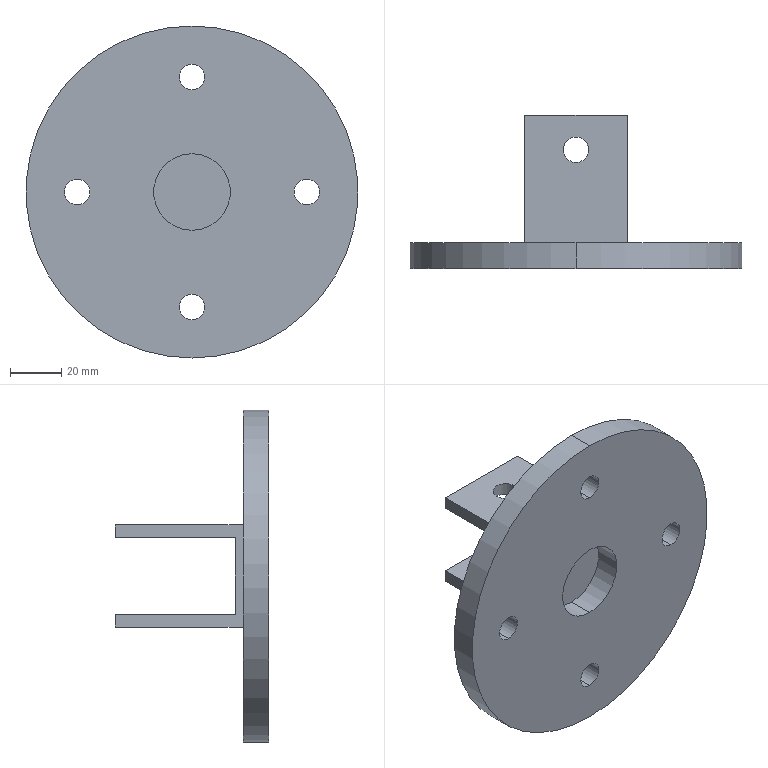Part | SolidWorks | features ICE 4, Extrusion 1 | 1 solid | 28 faces | box 130 x 60 x 130 mm | volume 145337 mm3 | cylinder 16 | plane 12 | commonest cylinder face diameters 10 x12 30 x2 130 x2
STEP:
#1=CARTESIAN_POINT('',(-5.,46.469,15.));
#2=VERTEX_POINT('',#1);
#3=CARTESIAN_POINT('',(5.,46.469,15.));
#4=VERTEX_POINT('',#3);
#5=CARTESIAN_POINT('',(0.,46.469,15.));
#6=DIRECTION('',(0.,0.,1.));
#7=DIRECTION('',(0.,-1.,0.));
#8=AXIS2_PLACEMENT_3D('',#5,#6,#7);
#9=CIRCLE('',#8,5.);
#10=EDGE_CURVE('',#2,#4,#9,.T.);
#11=ORIENTED_EDGE('',*,*,#10,.F.);
#12=CARTESIAN_POINT('',(-5.,46.469,20.));
#13=VERTEX_POINT('',#12);
#14=CARTESIAN_POINT('',(-5.,46.469,-65.));
#15=DIRECTION('',(0.,0.,1.));
#16=VECTOR('',#15,1000.);
#17=LINE('',#14,#16);
#18=EDGE_CURVE('',#2,#13,#17,.T.);
#19=ORIENTED_EDGE('',*,*,#18,.T.);
#20=CARTESIAN_POINT('',(5.,46.469,20.));
#21=VERTEX_POINT('',#20);
#22=CARTESIAN_POINT('',(0.,46.469,20.));
#23=DIRECTION('',(0.,0.,1.));
#24=DIRECTION('',(1.,0.,0.));
#25=AXIS2_PLACEMENT_3D('',#22,#23,#24);
#26=CIRCLE('',#25,5.);
#27=EDGE_CURVE('',#13,#21,#26,.T.);
#28=ORIENTED_EDGE('',*,*,#27,.T.);
#29=CARTESIAN_POINT('',(5.,46.469,-65.));
#30=DIRECTION('',(0.,0.,1.));
#31=VECTOR('',#30,1000.);
#32=LINE('',#29,#31);
#33=EDGE_CURVE('',#4,#21,#32,.T.);
#34=ORIENTED_EDGE('',*,*,#33,.F.);
#35=EDGE_LOOP('',(#11,#19,#28,#34));
#36=FACE_OUTER_BOUND('',#35,.T.);
#37=CARTESIAN_POINT('',(0.,46.469,-65.));
#38=DIRECTION('',(0.,0.,1.));
#39=DIRECTION('',(1.,0.,0.));
#40=AXIS2_PLACEMENT_3D('',#37,#38,#39);
#41=CYLINDRICAL_SURFACE('',#40,5.);
#42=ADVANCED_FACE('',(#36),#41,.F.);
#43=CARTESIAN_POINT('',(-5.,46.469,-20.));
#44=VERTEX_POINT('',#43);
#45=CARTESIAN_POINT('',(5.,46.469,-20.));
#46=VERTEX_POINT('',#45);
#47=CARTESIAN_POINT('',(0.,46.469,-20.));
#48=DIRECTION('',(0.,0.,1.));
#49=DIRECTION('',(1.,0.,0.));
#50=AXIS2_PLACEMENT_3D('',#47,#48,#49);
#51=CIRCLE('',#50,5.);
#52=EDGE_CURVE('',#44,#46,#51,.T.);
#53=ORIENTED_EDGE('',*,*,#52,.F.);
#54=CARTESIAN_POINT('',(-5.,46.469,-15.));
#55=VERTEX_POINT('',#54);
#56=CARTESIAN_POINT('',(-5.,46.469,-65.));
#57=DIRECTION('',(0.,0.,1.));
#58=VECTOR('',#57,1000.);
#59=LINE('',#56,#58);
#60=EDGE_CURVE('',#44,#55,#59,.T.);
#61=ORIENTED_EDGE('',*,*,#60,.T.);
#62=CARTESIAN_POINT('',(5.,46.469,-15.));
#63=VERTEX_POINT('',#62);
#64=CARTESIAN_POINT('',(0.,46.469,-15.));
#65=DIRECTION('',(0.,0.,-1.));
#66=DIRECTION('',(0.,1.,0.));
#67=AXIS2_PLACEMENT_3D('',#64,#65,#66);
#68=CIRCLE('',#67,5.);
#69=EDGE_CURVE('',#63,#55,#68,.T.);
#70=ORIENTED_EDGE('',*,*,#69,.F.);
#71=CARTESIAN_POINT('',(5.,46.469,-65.));
#72=DIRECTION('',(0.,0.,1.));
#73=VECTOR('',#72,1000.);
#74=LINE('',#71,#73);
#75=EDGE_CURVE('',#46,#63,#74,.T.);
#76=ORIENTED_EDGE('',*,*,#75,.F.);
#77=EDGE_LOOP('',(#53,#61,#70,#76));
#78=FACE_OUTER_BOUND('',#77,.T.);
#79=CARTESIAN_POINT('',(0.,46.469,-65.));
#80=DIRECTION('',(0.,0.,1.));
#81=DIRECTION('',(1.,0.,0.));
#82=AXIS2_PLACEMENT_3D('',#79,#80,#81);
#83=CYLINDRICAL_SURFACE('',#82,5.);
#84=ADVANCED_FACE('',(#78),#83,.F.);
#85=CARTESIAN_POINT('',(0.,0.,-50.));
#86=VERTEX_POINT('',#85);
#87=CARTESIAN_POINT('',(0.,0.,-40.));
#88=VERTEX_POINT('',#87);
#89=CARTESIAN_POINT('',(0.,0.,-45.));
#90=DIRECTION('',(0.,1.,0.));
#91=DIRECTION('',(0.,0.,1.));
#92=AXIS2_PLACEMENT_3D('',#89,#90,#91);
#93=CIRCLE('',#92,5.);
#94=EDGE_CURVE('',#86,#88,#93,.T.);
#95=ORIENTED_EDGE('',*,*,#94,.F.);
#96=CARTESIAN_POINT('',(0.,10.,-50.));
#97=VERTEX_POINT('',#96);
#98=CARTESIAN_POINT('',(0.,0.,-50.));
#99=DIRECTION('',(0.,1.,0.));
#100=VECTOR('',#99,1000.);
#101=LINE('',#98,#100);
#102=EDGE_CURVE('',#86,#97,#101,.T.);
#103=ORIENTED_EDGE('',*,*,#102,.T.);
#104=CARTESIAN_POINT('',(0.,10.,-40.));
#105=VERTEX_POINT('',#104);
#106=CARTESIAN_POINT('',(0.,10.,-45.));
#107=DIRECTION('',(0.,1.,0.));
#108=DIRECTION('',(0.,0.,1.));
#109=AXIS2_PLACEMENT_3D('',#106,#107,#108);
#110=CIRCLE('',#109,5.);
#111=EDGE_CURVE('',#97,#105,#110,.T.);
#112=ORIENTED_EDGE('',*,*,#111,.T.);
#113=CARTESIAN_POINT('',(0.,0.,-40.));
#114=DIRECTION('',(0.,1.,0.));
#115=VECTOR('',#114,1000.);
#116=LINE('',#113,#115);
#117=EDGE_CURVE('',#88,#105,#116,.T.);
#118=ORIENTED_EDGE('',*,*,#117,.F.);
#119=EDGE_LOOP('',(#95,#103,#112,#118));
#120=FACE_OUTER_BOUND('',#119,.T.);
#121=CARTESIAN_POINT('',(0.,0.,-45.));
#122=DIRECTION('',(0.,1.,0.));
#123=DIRECTION('',(0.,0.,1.));
#124=AXIS2_PLACEMENT_3D('',#121,#122,#123);
#125=CYLINDRICAL_SURFACE('',#124,5.);
#126=ADVANCED_FACE('',(#120),#125,.F.);
#127=CARTESIAN_POINT('',(45.,0.,-5.));
#128=VERTEX_POINT('',#127);
#129=CARTESIAN_POINT('',(45.,0.,5.));
#130=VERTEX_POINT('',#129);
#131=CARTESIAN_POINT('',(45.,0.,0.));
#132=DIRECTION('',(0.,1.,0.));
#133=DIRECTION('',(0.,0.,1.));
#134=AXIS2_PLACEMENT_3D('',#131,#132,#133);
#135=CIRCLE('',#134,5.);
#136=EDGE_CURVE('',#128,#130,#135,.T.);
#137=ORIENTED_EDGE('',*,*,#136,.F.);
#138=CARTESIAN_POINT('',(45.,10.,-5.));
#139=VERTEX_POINT('',#138);
#140=CARTESIAN_POINT('',(45.,0.,-5.));
#141=DIRECTION('',(0.,1.,0.));
#142=VECTOR('',#141,1000.);
#143=LINE('',#140,#142);
#144=EDGE_CURVE('',#128,#139,#143,.T.);
#145=ORIENTED_EDGE('',*,*,#144,.T.);
#146=CARTESIAN_POINT('',(45.,10.,5.));
#147=VERTEX_POINT('',#146);
#148=CARTESIAN_POINT('',(45.,10.,0.));
#149=DIRECTION('',(0.,1.,0.));
#150=DIRECTION('',(0.,0.,1.));
#151=AXIS2_PLACEMENT_3D('',#148,#149,#150);
#152=CIRCLE('',#151,5.);
#153=EDGE_CURVE('',#139,#147,#152,.T.);
#154=ORIENTED_EDGE('',*,*,#153,.T.);
#155=CARTESIAN_POINT('',(45.,0.,5.));
#156=DIRECTION('',(0.,1.,0.));
#157=VECTOR('',#156,1000.);
#158=LINE('',#155,#157);
#159=EDGE_CURVE('',#130,#147,#158,.T.);
#160=ORIENTED_EDGE('',*,*,#159,.F.);
#161=EDGE_LOOP('',(#137,#145,#154,#160));
#162=FACE_OUTER_BOUND('',#161,.T.);
#163=CARTESIAN_POINT('',(45.,0.,0.));
#164=DIRECTION('',(0.,1.,0.));
#165=DIRECTION('',(0.,0.,1.));
#166=AXIS2_PLACEMENT_3D('',#163,#164,#165);
#167=CYLINDRICAL_SURFACE('',#166,5.);
#168=ADVANCED_FACE('',(#162),#167,.F.);
#169=CARTESIAN_POINT('',(0.,0.,40.));
#170=VERTEX_POINT('',#169);
#171=CARTESIAN_POINT('',(0.,0.,50.));
#172=VERTEX_POINT('',#171);
#173=CARTESIAN_POINT('',(0.,0.,45.));
#174=DIRECTION('',(0.,1.,0.));
#175=DIRECTION('',(0.,0.,1.));
#176=AXIS2_PLACEMENT_3D('',#173,#174,#175);
#177=CIRCLE('',#176,5.);
#178=EDGE_CURVE('',#170,#172,#177,.T.);
#179=ORIENTED_EDGE('',*,*,#178,.F.);
#180=CARTESIAN_POINT('',(0.,10.,40.));
#181=VERTEX_POINT('',#180);
#182=CARTESIAN_POINT('',(0.,0.,40.));
#183=DIRECTION('',(0.,1.,0.));
#184=VECTOR('',#183,1000.);
#185=LINE('',#182,#184);
#186=EDGE_CURVE('',#170,#181,#185,.T.);
#187=ORIENTED_EDGE('',*,*,#186,.T.);
#188=CARTESIAN_POINT('',(0.,10.,50.));
#189=VERTEX_POINT('',#188);
#190=CARTESIAN_POINT('',(0.,10.,45.));
#191=DIRECTION('',(0.,1.,0.));
#192=DIRECTION('',(0.,0.,1.));
#193=AXIS2_PLACEMENT_3D('',#190,#191,#192);
#194=CIRCLE('',#193,5.);
#195=EDGE_CURVE('',#181,#189,#194,.T.);
#196=ORIENTED_EDGE('',*,*,#195,.T.);
#197=CARTESIAN_POINT('',(0.,0.,50.));
#198=DIRECTION('',(0.,1.,0.));
#199=VECTOR('',#198,1000.);
#200=LINE('',#197,#199);
#201=EDGE_CURVE('',#172,#189,#200,.T.);
#202=ORIENTED_EDGE('',*,*,#201,.F.);
#203=EDGE_LOOP('',(#179,#187,#196,#202));
#204=FACE_OUTER_BOUND('',#203,.T.);
#205=CARTESIAN_POINT('',(0.,0.,45.));
#206=DIRECTION('',(0.,1.,0.));
#207=DIRECTION('',(0.,0.,1.));
#208=AXIS2_PLACEMENT_3D('',#205,#206,#207);
#209=CYLINDRICAL_SURFACE('',#208,5.);
#210=ADVANCED_FACE('',(#204),#209,.F.);
#211=CARTESIAN_POINT('',(-45.,0.,-5.));
#212=VERTEX_POINT('',#211);
#213=CARTESIAN_POINT('',(-45.,0.,5.));
#214=VERTEX_POINT('',#213);
#215=CARTESIAN_POINT('',(-45.,0.,0.));
#216=DIRECTION('',(0.,1.,0.));
#217=DIRECTION('',(0.,0.,1.));
#218=AXIS2_PLACEMENT_3D('',#215,#216,#217);
#219=CIRCLE('',#218,5.);
#220=EDGE_CURVE('',#212,#214,#219,.T.);
#221=ORIENTED_EDGE('',*,*,#220,.F.);
#222=CARTESIAN_POINT('',(-45.,10.,-5.));
#223=VERTEX_POINT('',#222);
#224=CARTESIAN_POINT('',(-45.,0.,-5.));
#225=DIRECTION('',(0.,1.,0.));
#226=VECTOR('',#225,1000.);
#227=LINE('',#224,#226);
#228=EDGE_CURVE('',#212,#223,#227,.T.);
#229=ORIENTED_EDGE('',*,*,#228,.T.);
#230=CARTESIAN_POINT('',(-45.,10.,5.));
#231=VERTEX_POINT('',#230);
#232=CARTESIAN_POINT('',(-45.,10.,0.));
#233=DIRECTION('',(0.,1.,0.));
#234=DIRECTION('',(0.,0.,1.));
#235=AXIS2_PLACEMENT_3D('',#232,#233,#234);
#236=CIRCLE('',#235,5.);
#237=EDGE_CURVE('',#223,#231,#236,.T.);
#238=ORIENTED_EDGE('',*,*,#237,.T.);
#239=CARTESIAN_POINT('',(-45.,0.,5.));
#240=DIRECTION('',(0.,1.,0.));
#241=VECTOR('',#240,1000.);
#242=LINE('',#239,#241);
#243=EDGE_CURVE('',#214,#231,#242,.T.);
#244=ORIENTED_EDGE('',*,*,#243,.F.);
#245=EDGE_LOOP('',(#221,#229,#238,#244));
#246=FACE_OUTER_BOUND('',#245,.T.);
#247=CARTESIAN_POINT('',(-45.,0.,0.));
#248=DIRECTION('',(0.,1.,0.));
#249=DIRECTION('',(0.,0.,1.));
#250=AXIS2_PLACEMENT_3D('',#247,#248,#249);
#251=CYLINDRICAL_SURFACE('',#250,5.);
#252=ADVANCED_FACE('',(#246),#251,.F.);
#253=CARTESIAN_POINT('',(0.,10.,15.));
#254=VERTEX_POINT('',#253);
#255=CARTESIAN_POINT('',(0.,10.,-15.));
#256=VERTEX_POINT('',#255);
#257=CARTESIAN_POINT('',(0.,10.,0.));
#258=DIRECTION('',(0.,-1.,0.));
#259=DIRECTION('',(0.,0.,-1.));
#260=AXIS2_PLACEMENT_3D('',#257,#258,#259);
#261=CIRCLE('',#260,15.);
#262=EDGE_CURVE('',#254,#256,#261,.T.);
#263=ORIENTED_EDGE('',*,*,#262,.F.);
#264=CARTESIAN_POINT('',(0.,0.,15.));
#265=VERTEX_POINT('',#264);
#266=CARTESIAN_POINT('',(0.,10.,15.));
#267=DIRECTION('',(0.,-1.,0.));
#268=VECTOR('',#267,1000.);
#269=LINE('',#266,#268);
#270=EDGE_CURVE('',#254,#265,#269,.T.);
#271=ORIENTED_EDGE('',*,*,#270,.T.);
#272=CARTESIAN_POINT('',(0.,0.,-15.));
#273=VERTEX_POINT('',#272);
#274=CARTESIAN_POINT('',(0.,0.,0.));
#275=DIRECTION('',(0.,1.,0.));
#276=DIRECTION('',(0.,0.,1.));
#277=AXIS2_PLACEMENT_3D('',#274,#275,#276);
#278=CIRCLE('',#277,15.);
#279=EDGE_CURVE('',#273,#265,#278,.T.);
#280=ORIENTED_EDGE('',*,*,#279,.F.);
#281=CARTESIAN_POINT('',(0.,10.,-15.));
#282=DIRECTION('',(0.,-1.,0.));
#283=VECTOR('',#282,1000.);
#284=LINE('',#281,#283);
#285=EDGE_CURVE('',#256,#273,#284,.T.);
#286=ORIENTED_EDGE('',*,*,#285,.F.);
#287=EDGE_LOOP('',(#263,#271,#280,#286));
#288=FACE_OUTER_BOUND('',#287,.T.);
#289=CARTESIAN_POINT('',(0.,10.,0.));
#290=DIRECTION('',(0.,-1.,0.));
#291=DIRECTION('',(0.,0.,-1.));
#292=AXIS2_PLACEMENT_3D('',#289,#290,#291);
#293=CYLINDRICAL_SURFACE('',#292,15.);
#294=ADVANCED_FACE('',(#288),#293,.F.);
#295=CARTESIAN_POINT('',(0.,10.,65.));
#296=VERTEX_POINT('',#295);
#297=CARTESIAN_POINT('',(0.,10.,-65.));
#298=VERTEX_POINT('',#297);
#299=CARTESIAN_POINT('',(0.,10.,0.));
#300=DIRECTION('',(0.,1.,0.));
#301=DIRECTION('',(0.,0.,1.));
#302=AXIS2_PLACEMENT_3D('',#299,#300,#301);
#303=CIRCLE('',#302,65.);
#304=EDGE_CURVE('',#296,#298,#303,.T.);
#305=ORIENTED_EDGE('',*,*,#304,.F.);
#306=CARTESIAN_POINT('',(0.,0.,65.));
#307=VERTEX_POINT('',#306);
#308=CARTESIAN_POINT('',(0.,10.,65.));
#309=DIRECTION('',(0.,-1.,0.));
#310=VECTOR('',#309,1000.);
#311=LINE('',#308,#310);
#312=EDGE_CURVE('',#296,#307,#311,.T.);
#313=ORIENTED_EDGE('',*,*,#312,.T.);
#314=CARTESIAN_POINT('',(0.,0.,-65.));
#315=VERTEX_POINT('',#314);
#316=CARTESIAN_POINT('',(0.,0.,0.));
#317=DIRECTION('',(0.,1.,0.));
#318=DIRECTION('',(0.,0.,1.));
#319=AXIS2_PLACEMENT_3D('',#316,#317,#318);
#320=CIRCLE('',#319,65.);
#321=EDGE_CURVE('',#307,#315,#320,.T.);
#322=ORIENTED_EDGE('',*,*,#321,.T.);
#323=CARTESIAN_POINT('',(0.,10.,-65.));
#324=DIRECTION('',(0.,-1.,0.));
#325=VECTOR('',#324,1000.);
#326=LINE('',#323,#325);
#327=EDGE_CURVE('',#298,#315,#326,.T.);
#328=ORIENTED_EDGE('',*,*,#327,.F.);
#329=EDGE_LOOP('',(#305,#313,#322,#328));
#330=FACE_OUTER_BOUND('',#329,.T.);
#331=CARTESIAN_POINT('',(0.,10.,0.));
#332=DIRECTION('',(0.,-1.,0.));
#333=DIRECTION('',(0.,0.,-1.));
#334=AXIS2_PLACEMENT_3D('',#331,#332,#333);
#335=CYLINDRICAL_SURFACE('',#334,65.);
#336=ADVANCED_FACE('',(#330),#335,.T.);
#337=CARTESIAN_POINT('',(20.,60.,20.));
#338=VERTEX_POINT('',#337);
#339=CARTESIAN_POINT('',(20.,60.,15.));
#340=VERTEX_POINT('',#339);
#341=CARTESIAN_POINT('',(20.,60.,20.));
#342=DIRECTION('',(0.,0.,-1.));
#343=VECTOR('',#342,1000.);
#344=LINE('',#341,#343);
#345=EDGE_CURVE('',#338,#340,#344,.T.);
#346=ORIENTED_EDGE('',*,*,#345,.T.);
#347=CARTESIAN_POINT('',(-20.,60.,15.));
#348=VERTEX_POINT('',#347);
#349=CARTESIAN_POINT('',(0.,60.,15.));
#350=DIRECTION('',(-1.,0.,0.));
#351=VECTOR('',#350,1000.);
#352=LINE('',#349,#351);
#353=EDGE_CURVE('',#340,#348,#352,.T.);
#354=ORIENTED_EDGE('',*,*,#353,.T.);
#355=CARTESIAN_POINT('',(-20.,60.,20.));
#356=VERTEX_POINT('',#355);
#357=CARTESIAN_POINT('',(-20.,60.,20.));
#358=DIRECTION('',(0.,0.,1.));
#359=VECTOR('',#358,1000.);
#360=LINE('',#357,#359);
#361=EDGE_CURVE('',#348,#356,#360,.T.);
#362=ORIENTED_EDGE('',*,*,#361,.T.);
#363=CARTESIAN_POINT('',(-20.,60.,20.));
#364=DIRECTION('',(1.,0.,0.));
#365=VECTOR('',#364,1000.);
#366=LINE('',#363,#365);
#367=EDGE_CURVE('',#356,#338,#366,.T.);
#368=ORIENTED_EDGE('',*,*,#367,.T.);
#369=EDGE_LOOP('',(#346,#354,#362,#368));
#370=FACE_OUTER_BOUND('',#369,.T.);
#371=CARTESIAN_POINT('',(0.,60.,0.));
#372=DIRECTION('',(0.,-1.,0.));
#373=DIRECTION('',(0.,0.,-1.));
#374=AXIS2_PLACEMENT_3D('',#371,#372,#373);
#375=PLANE('',#374);
#376=ADVANCED_FACE('',(#370),#375,.F.);
#377=CARTESIAN_POINT('',(0.,10.,0.));
#378=DIRECTION('',(0.,1.,0.));
#379=DIRECTION('',(0.,0.,1.));
#380=AXIS2_PLACEMENT_3D('',#377,#378,#379);
#381=CIRCLE('',#380,65.);
#382=EDGE_CURVE('',#298,#296,#381,.T.);
#383=ORIENTED_EDGE('',*,*,#382,.T.);
#384=ORIENTED_EDGE('',*,*,#304,.T.);
#385=EDGE_LOOP('',(#383,#384));
#386=FACE_OUTER_BOUND('',#385,.T.);
#387=CARTESIAN_POINT('',(-45.,10.,0.));
#388=DIRECTION('',(0.,1.,0.));
#389=DIRECTION('',(0.,0.,1.));
#390=AXIS2_PLACEMENT_3D('',#387,#388,#389);
#391=CIRCLE('',#390,5.);
#392=EDGE_CURVE('',#231,#223,#391,.T.);
#393=ORIENTED_EDGE('',*,*,#392,.F.);
#394=ORIENTED_EDGE('',*,*,#237,.F.);
#395=EDGE_LOOP('',(#393,#394));
#396=FACE_BOUND('',#395,.T.);
#397=CARTESIAN_POINT('',(0.,10.,45.));
#398=DIRECTION('',(0.,1.,0.));
#399=DIRECTION('',(0.,0.,1.));
#400=AXIS2_PLACEMENT_3D('',#397,#398,#399);
#401=CIRCLE('',#400,5.);
#402=EDGE_CURVE('',#189,#181,#401,.T.);
#403=ORIENTED_EDGE('',*,*,#402,.F.);
#404=ORIENTED_EDGE('',*,*,#195,.F.);
#405=EDGE_LOOP('',(#403,#404));
#406=FACE_BOUND('',#405,.T.);
#407=CARTESIAN_POINT('',(45.,10.,0.));
#408=DIRECTION('',(0.,1.,0.));
#409=DIRECTION('',(0.,0.,1.));
#410=AXIS2_PLACEMENT_3D('',#407,#408,#409);
#411=CIRCLE('',#410,5.);
#412=EDGE_CURVE('',#147,#139,#411,.T.);
#413=ORIENTED_EDGE('',*,*,#412,.F.);
#414=ORIENTED_EDGE('',*,*,#153,.F.);
#415=EDGE_LOOP('',(#413,#414));
#416=FACE_BOUND('',#415,.T.);
#417=CARTESIAN_POINT('',(0.,10.,-45.));
#418=DIRECTION('',(0.,1.,0.));
#419=DIRECTION('',(0.,0.,1.));
#420=AXIS2_PLACEMENT_3D('',#417,#418,#419);
#421=CIRCLE('',#420,5.);
#422=EDGE_CURVE('',#105,#97,#421,.T.);
#423=ORIENTED_EDGE('',*,*,#422,.F.);
#424=ORIENTED_EDGE('',*,*,#111,.F.);
#425=EDGE_LOOP('',(#423,#424));
#426=FACE_BOUND('',#425,.T.);
#427=CARTESIAN_POINT('',(20.,10.,-20.));
#428=VERTEX_POINT('',#427);
#429=CARTESIAN_POINT('',(-20.,10.,-20.));
#430=VERTEX_POINT('',#429);
#431=CARTESIAN_POINT('',(-20.,10.,-20.));
#432=DIRECTION('',(-1.,0.,0.));
#433=VECTOR('',#432,1000.);
#434=LINE('',#431,#433);
#435=EDGE_CURVE('',#428,#430,#434,.T.);
#436=ORIENTED_EDGE('',*,*,#435,.F.);
#437=CARTESIAN_POINT('',(20.,10.,20.));
#438=VERTEX_POINT('',#437);
#439=CARTESIAN_POINT('',(20.,10.,20.));
#440=DIRECTION('',(0.,0.,-1.));
#441=VECTOR('',#440,1000.);
#442=LINE('',#439,#441);
#443=EDGE_CURVE('',#438,#428,#442,.T.);
#444=ORIENTED_EDGE('',*,*,#443,.F.);
#445=CARTESIAN_POINT('',(-20.,10.,20.));
#446=VERTEX_POINT('',#445);
#447=CARTESIAN_POINT('',(-20.,10.,20.));
#448=DIRECTION('',(1.,0.,0.));
#449=VECTOR('',#448,1000.);
#450=LINE('',#447,#449);
#451=EDGE_CURVE('',#446,#438,#450,.T.);
#452=ORIENTED_EDGE('',*,*,#451,.F.);
#453=CARTESIAN_POINT('',(-20.,10.,20.));
#454=DIRECTION('',(0.,0.,1.));
#455=VECTOR('',#454,1000.);
#456=LINE('',#453,#455);
#457=EDGE_CURVE('',#430,#446,#456,.T.);
#458=ORIENTED_EDGE('',*,*,#457,.F.);
#459=EDGE_LOOP('',(#436,#444,#452,#458));
#460=FACE_BOUND('',#459,.T.);
#461=CARTESIAN_POINT('',(0.,10.,0.));
#462=DIRECTION('',(0.,1.,0.));
#463=DIRECTION('',(0.,0.,1.));
#464=AXIS2_PLACEMENT_3D('',#461,#462,#463);
#465=PLANE('',#464);
#466=ADVANCED_FACE('',(#386,#396,#406,#416,#426,#460),#465,.T.);
#467=CARTESIAN_POINT('',(0.,0.,-45.));
#468=DIRECTION('',(0.,1.,0.));
#469=DIRECTION('',(0.,0.,1.));
#470=AXIS2_PLACEMENT_3D('',#467,#468,#469);
#471=CIRCLE('',#470,5.);
#472=EDGE_CURVE('',#88,#86,#471,.T.);
#473=ORIENTED_EDGE('',*,*,#472,.T.);
#474=ORIENTED_EDGE('',*,*,#94,.T.);
#475=EDGE_LOOP('',(#473,#474));
#476=FACE_BOUND('',#475,.T.);
#477=CARTESIAN_POINT('',(45.,0.,0.));
#478=DIRECTION('',(0.,1.,0.));
#479=DIRECTION('',(0.,0.,1.));
#480=AXIS2_PLACEMENT_3D('',#477,#478,#479);
#481=CIRCLE('',#480,5.);
#482=EDGE_CURVE('',#130,#128,#481,.T.);
#483=ORIENTED_EDGE('',*,*,#482,.T.);
#484=ORIENTED_EDGE('',*,*,#136,.T.);
#485=EDGE_LOOP('',(#483,#484));
#486=FACE_BOUND('',#485,.T.);
#487=CARTESIAN_POINT('',(0.,0.,45.));
#488=DIRECTION('',(0.,1.,0.));
#489=DIRECTION('',(0.,0.,1.));
#490=AXIS2_PLACEMENT_3D('',#487,#488,#489);
#491=CIRCLE('',#490,5.);
#492=EDGE_CURVE('',#172,#170,#491,.T.);
#493=ORIENTED_EDGE('',*,*,#492,.T.);
#494=ORIENTED_EDGE('',*,*,#178,.T.);
#495=EDGE_LOOP('',(#493,#494));
#496=FACE_BOUND('',#495,.T.);
#497=CARTESIAN_POINT('',(-45.,0.,0.));
#498=DIRECTION('',(0.,1.,0.));
#499=DIRECTION('',(0.,0.,1.));
#500=AXIS2_PLACEMENT_3D('',#497,#498,#499);
#501=CIRCLE('',#500,5.);
#502=EDGE_CURVE('',#214,#212,#501,.T.);
#503=ORIENTED_EDGE('',*,*,#502,.T.);
#504=ORIENTED_EDGE('',*,*,#220,.T.);
#505=EDGE_LOOP('',(#503,#504));
#506=FACE_BOUND('',#505,.T.);
#507=CARTESIAN_POINT('',(0.,0.,0.));
#508=DIRECTION('',(0.,1.,0.));
#509=DIRECTION('',(0.,0.,1.));
#510=AXIS2_PLACEMENT_3D('',#507,#508,#509);
#511=CIRCLE('',#510,65.);
#512=EDGE_CURVE('',#315,#307,#511,.T.);
#513=ORIENTED_EDGE('',*,*,#512,.F.);
#514=ORIENTED_EDGE('',*,*,#321,.F.);
#515=EDGE_LOOP('',(#513,#514));
#516=FACE_OUTER_BOUND('',#515,.T.);
#517=ORIENTED_EDGE('',*,*,#279,.T.);
#518=CARTESIAN_POINT('',(0.,0.,0.));
#519=DIRECTION('',(0.,1.,0.));
#520=DIRECTION('',(0.,0.,1.));
#521=AXIS2_PLACEMENT_3D('',#518,#519,#520);
#522=CIRCLE('',#521,15.);
#523=EDGE_CURVE('',#265,#273,#522,.T.);
#524=ORIENTED_EDGE('',*,*,#523,.T.);
#525=EDGE_LOOP('',(#517,#524));
#526=FACE_BOUND('',#525,.T.);
#527=CARTESIAN_POINT('',(0.,0.,0.));
#528=DIRECTION('',(0.,1.,0.));
#529=DIRECTION('',(0.,0.,1.));
#530=AXIS2_PLACEMENT_3D('',#527,#528,#529);
#531=PLANE('',#530);
#532=ADVANCED_FACE('',(#476,#486,#496,#506,#516,#526),#531,.F.);
#533=ORIENTED_EDGE('',*,*,#312,.F.);
#534=ORIENTED_EDGE('',*,*,#382,.F.);
#535=ORIENTED_EDGE('',*,*,#327,.T.);
#536=ORIENTED_EDGE('',*,*,#512,.T.);
#537=EDGE_LOOP('',(#533,#534,#535,#536));
#538=FACE_OUTER_BOUND('',#537,.T.);
#539=CARTESIAN_POINT('',(0.,10.,0.));
#540=DIRECTION('',(0.,-1.,0.));
#541=DIRECTION('',(0.,0.,-1.));
#542=AXIS2_PLACEMENT_3D('',#539,#540,#541);
#543=CYLINDRICAL_SURFACE('',#542,65.);
#544=ADVANCED_FACE('',(#538),#543,.T.);
#545=ORIENTED_EDGE('',*,*,#270,.F.);
#546=CARTESIAN_POINT('',(0.,10.,0.));
#547=DIRECTION('',(0.,-1.,0.));
#548=DIRECTION('',(0.,0.,-1.));
#549=AXIS2_PLACEMENT_3D('',#546,#547,#548);
#550=CIRCLE('',#549,15.);
#551=EDGE_CURVE('',#256,#254,#550,.T.);
#552=ORIENTED_EDGE('',*,*,#551,.F.);
#553=ORIENTED_EDGE('',*,*,#285,.T.);
#554=ORIENTED_EDGE('',*,*,#523,.F.);
#555=EDGE_LOOP('',(#545,#552,#553,#554));
#556=FACE_OUTER_BOUND('',#555,.T.);
#557=CARTESIAN_POINT('',(0.,10.,0.));
#558=DIRECTION('',(0.,-1.,0.));
#559=DIRECTION('',(0.,0.,-1.));
#560=AXIS2_PLACEMENT_3D('',#557,#558,#559);
#561=CYLINDRICAL_SURFACE('',#560,15.);
#562=ADVANCED_FACE('',(#556),#561,.F.);
#563=ORIENTED_EDGE('',*,*,#228,.F.);
#564=ORIENTED_EDGE('',*,*,#502,.F.);
#565=ORIENTED_EDGE('',*,*,#243,.T.);
#566=ORIENTED_EDGE('',*,*,#392,.T.);
#567=EDGE_LOOP('',(#563,#564,#565,#566));
#568=FACE_OUTER_BOUND('',#567,.T.);
#569=CARTESIAN_POINT('',(-45.,0.,0.));
#570=DIRECTION('',(0.,1.,0.));
#571=DIRECTION('',(0.,0.,1.));
#572=AXIS2_PLACEMENT_3D('',#569,#570,#571);
#573=CYLINDRICAL_SURFACE('',#572,5.);
#574=ADVANCED_FACE('',(#568),#573,.F.);
#575=ORIENTED_EDGE('',*,*,#186,.F.);
#576=ORIENTED_EDGE('',*,*,#492,.F.);
#577=ORIENTED_EDGE('',*,*,#201,.T.);
#578=ORIENTED_EDGE('',*,*,#402,.T.);
#579=EDGE_LOOP('',(#575,#576,#577,#578));
#580=FACE_OUTER_BOUND('',#579,.T.);
#581=CARTESIAN_POINT('',(0.,0.,45.));
#582=DIRECTION('',(0.,1.,0.));
#583=DIRECTION('',(0.,0.,1.));
#584=AXIS2_PLACEMENT_3D('',#581,#582,#583);
#585=CYLINDRICAL_SURFACE('',#584,5.);
#586=ADVANCED_FACE('',(#580),#585,.F.);
#587=ORIENTED_EDGE('',*,*,#144,.F.);
#588=ORIENTED_EDGE('',*,*,#482,.F.);
#589=ORIENTED_EDGE('',*,*,#159,.T.);
#590=ORIENTED_EDGE('',*,*,#412,.T.);
#591=EDGE_LOOP('',(#587,#588,#589,#590));
#592=FACE_OUTER_BOUND('',#591,.T.);
#593=CARTESIAN_POINT('',(45.,0.,0.));
#594=DIRECTION('',(0.,1.,0.));
#595=DIRECTION('',(0.,0.,1.));
#596=AXIS2_PLACEMENT_3D('',#593,#594,#595);
#597=CYLINDRICAL_SURFACE('',#596,5.);
#598=ADVANCED_FACE('',(#592),#597,.F.);
#599=ORIENTED_EDGE('',*,*,#102,.F.);
#600=ORIENTED_EDGE('',*,*,#472,.F.);
#601=ORIENTED_EDGE('',*,*,#117,.T.);
#602=ORIENTED_EDGE('',*,*,#422,.T.);
#603=EDGE_LOOP('',(#599,#600,#601,#602));
#604=FACE_OUTER_BOUND('',#603,.T.);
#605=CARTESIAN_POINT('',(0.,0.,-45.));
#606=DIRECTION('',(0.,1.,0.));
#607=DIRECTION('',(0.,0.,1.));
#608=AXIS2_PLACEMENT_3D('',#605,#606,#607);
#609=CYLINDRICAL_SURFACE('',#608,5.);
#610=ADVANCED_FACE('',(#604),#609,.F.);
#611=ORIENTED_EDGE('',*,*,#551,.T.);
#612=ORIENTED_EDGE('',*,*,#262,.T.);
#613=EDGE_LOOP('',(#611,#612));
#614=FACE_OUTER_BOUND('',#613,.T.);
#615=CARTESIAN_POINT('',(0.,10.,0.));
#616=DIRECTION('',(0.,-1.,0.));
#617=DIRECTION('',(0.,0.,-1.));
#618=AXIS2_PLACEMENT_3D('',#615,#616,#617);
#619=PLANE('',#618);
#620=ADVANCED_FACE('',(#614),#619,.T.);
#621=CARTESIAN_POINT('',(20.,13.,15.));
#622=VERTEX_POINT('',#621);
#623=CARTESIAN_POINT('',(20.,13.,-15.));
#624=VERTEX_POINT('',#623);
#625=CARTESIAN_POINT('',(20.,13.,15.));
#626=DIRECTION('',(0.,0.,-1.));
#627=VECTOR('',#626,1000.);
#628=LINE('',#625,#627);
#629=EDGE_CURVE('',#622,#624,#628,.T.);
#630=ORIENTED_EDGE('',*,*,#629,.F.);
#631=CARTESIAN_POINT('',(20.,60.,15.));
#632=DIRECTION('',(0.,-1.,0.));
#633=VECTOR('',#632,1000.);
#634=LINE('',#631,#633);
#635=EDGE_CURVE('',#340,#622,#634,.T.);
#636=ORIENTED_EDGE('',*,*,#635,.F.);
#637=ORIENTED_EDGE('',*,*,#345,.F.);
#638=CARTESIAN_POINT('',(20.,60.,20.));
#639=DIRECTION('',(0.,-1.,0.));
#640=VECTOR('',#639,1000.);
#641=LINE('',#638,#640);
#642=EDGE_CURVE('',#338,#438,#641,.T.);
#643=ORIENTED_EDGE('',*,*,#642,.T.);
#644=ORIENTED_EDGE('',*,*,#443,.T.);
#645=CARTESIAN_POINT('',(20.,60.,-20.));
#646=VERTEX_POINT('',#645);
#647=CARTESIAN_POINT('',(20.,60.,-20.));
#648=DIRECTION('',(0.,-1.,0.));
#649=VECTOR('',#648,1000.);
#650=LINE('',#647,#649);
#651=EDGE_CURVE('',#646,#428,#650,.T.);
#652=ORIENTED_EDGE('',*,*,#651,.F.);
#653=CARTESIAN_POINT('',(20.,60.,-15.));
#654=VERTEX_POINT('',#653);
#655=CARTESIAN_POINT('',(20.,60.,20.));
#656=DIRECTION('',(0.,0.,-1.));
#657=VECTOR('',#656,1000.);
#658=LINE('',#655,#657);
#659=EDGE_CURVE('',#654,#646,#658,.T.);
#660=ORIENTED_EDGE('',*,*,#659,.F.);
#661=CARTESIAN_POINT('',(20.,60.,-15.));
#662=DIRECTION('',(0.,1.,0.));
#663=VECTOR('',#662,1000.);
#664=LINE('',#661,#663);
#665=EDGE_CURVE('',#624,#654,#664,.T.);
#666=ORIENTED_EDGE('',*,*,#665,.F.);
#667=EDGE_LOOP('',(#630,#636,#637,#643,#644,#652,#660,#666));
#668=FACE_OUTER_BOUND('',#667,.T.);
#669=CARTESIAN_POINT('',(20.,60.,20.));
#670=DIRECTION('',(-1.,0.,0.));
#671=DIRECTION('',(0.,0.,1.));
#672=AXIS2_PLACEMENT_3D('',#669,#670,#671);
#673=PLANE('',#672);
#674=ADVANCED_FACE('',(#668),#673,.F.);
#675=CARTESIAN_POINT('',(0.,46.469,-20.));
#676=DIRECTION('',(0.,0.,1.));
#677=DIRECTION('',(1.,0.,0.));
#678=AXIS2_PLACEMENT_3D('',#675,#676,#677);
#679=CIRCLE('',#678,5.);
#680=EDGE_CURVE('',#46,#44,#679,.T.);
#681=ORIENTED_EDGE('',*,*,#680,.T.);
#682=ORIENTED_EDGE('',*,*,#52,.T.);
#683=EDGE_LOOP('',(#681,#682));
#684=FACE_BOUND('',#683,.T.);
#685=ORIENTED_EDGE('',*,*,#435,.T.);
#686=CARTESIAN_POINT('',(-20.,60.,-20.));
#687=VERTEX_POINT('',#686);
#688=CARTESIAN_POINT('',(-20.,60.,-20.));
#689=DIRECTION('',(0.,-1.,0.));
#690=VECTOR('',#689,1000.);
#691=LINE('',#688,#690);
#692=EDGE_CURVE('',#687,#430,#691,.T.);
#693=ORIENTED_EDGE('',*,*,#692,.F.);
#694=CARTESIAN_POINT('',(-20.,60.,-20.));
#695=DIRECTION('',(-1.,0.,0.));
#696=VECTOR('',#695,1000.);
#697=LINE('',#694,#696);
#698=EDGE_CURVE('',#646,#687,#697,.T.);
#699=ORIENTED_EDGE('',*,*,#698,.F.);
#700=ORIENTED_EDGE('',*,*,#651,.T.);
#701=EDGE_LOOP('',(#685,#693,#699,#700));
#702=FACE_OUTER_BOUND('',#701,.T.);
#703=CARTESIAN_POINT('',(-20.,60.,-20.));
#704=DIRECTION('',(0.,0.,1.));
#705=DIRECTION('',(1.,0.,0.));
#706=AXIS2_PLACEMENT_3D('',#703,#704,#705);
#707=PLANE('',#706);
#708=ADVANCED_FACE('',(#684,#702),#707,.F.);
#709=ORIENTED_EDGE('',*,*,#361,.F.);
#710=CARTESIAN_POINT('',(-20.,13.,15.));
#711=VERTEX_POINT('',#710);
#712=CARTESIAN_POINT('',(-20.,60.,15.));
#713=DIRECTION('',(0.,-1.,0.));
#714=VECTOR('',#713,1000.);
#715=LINE('',#712,#714);
#716=EDGE_CURVE('',#348,#711,#715,.T.);
#717=ORIENTED_EDGE('',*,*,#716,.T.);
#718=CARTESIAN_POINT('',(-20.,13.,-15.));
#719=VERTEX_POINT('',#718);
#720=CARTESIAN_POINT('',(-20.,13.,20.));
#721=DIRECTION('',(0.,0.,-1.));
#722=VECTOR('',#721,1000.);
#723=LINE('',#720,#722);
#724=EDGE_CURVE('',#711,#719,#723,.T.);
#725=ORIENTED_EDGE('',*,*,#724,.T.);
#726=CARTESIAN_POINT('',(-20.,60.,-15.));
#727=VERTEX_POINT('',#726);
#728=CARTESIAN_POINT('',(-20.,60.,-15.));
#729=DIRECTION('',(0.,1.,0.));
#730=VECTOR('',#729,1000.);
#731=LINE('',#728,#730);
#732=EDGE_CURVE('',#719,#727,#731,.T.);
#733=ORIENTED_EDGE('',*,*,#732,.T.);
#734=CARTESIAN_POINT('',(-20.,60.,20.));
#735=DIRECTION('',(0.,0.,1.));
#736=VECTOR('',#735,1000.);
#737=LINE('',#734,#736);
#738=EDGE_CURVE('',#687,#727,#737,.T.);
#739=ORIENTED_EDGE('',*,*,#738,.F.);
#740=ORIENTED_EDGE('',*,*,#692,.T.);
#741=ORIENTED_EDGE('',*,*,#457,.T.);
#742=CARTESIAN_POINT('',(-20.,60.,20.));
#743=DIRECTION('',(0.,-1.,0.));
#744=VECTOR('',#743,1000.);
#745=LINE('',#742,#744);
#746=EDGE_CURVE('',#356,#446,#745,.T.);
#747=ORIENTED_EDGE('',*,*,#746,.F.);
#748=EDGE_LOOP('',(#709,#717,#725,#733,#739,#740,#741,#747));
#749=FACE_OUTER_BOUND('',#748,.T.);
#750=CARTESIAN_POINT('',(-20.,60.,20.));
#751=DIRECTION('',(1.,0.,0.));
#752=DIRECTION('',(0.,0.,-1.));
#753=AXIS2_PLACEMENT_3D('',#750,#751,#752);
#754=PLANE('',#753);
#755=ADVANCED_FACE('',(#749),#754,.F.);
#756=CARTESIAN_POINT('',(0.,46.469,20.));
#757=DIRECTION('',(0.,0.,1.));
#758=DIRECTION('',(1.,0.,0.));
#759=AXIS2_PLACEMENT_3D('',#756,#757,#758);
#760=CIRCLE('',#759,5.);
#761=EDGE_CURVE('',#21,#13,#760,.T.);
#762=ORIENTED_EDGE('',*,*,#761,.F.);
#763=ORIENTED_EDGE('',*,*,#27,.F.);
#764=EDGE_LOOP('',(#762,#763));
#765=FACE_BOUND('',#764,.T.);
#766=ORIENTED_EDGE('',*,*,#451,.T.);
#767=ORIENTED_EDGE('',*,*,#642,.F.);
#768=ORIENTED_EDGE('',*,*,#367,.F.);
#769=ORIENTED_EDGE('',*,*,#746,.T.);
#770=EDGE_LOOP('',(#766,#767,#768,#769));
#771=FACE_OUTER_BOUND('',#770,.T.);
#772=CARTESIAN_POINT('',(-20.,60.,20.));
#773=DIRECTION('',(0.,0.,-1.));
#774=DIRECTION('',(-1.,0.,0.));
#775=AXIS2_PLACEMENT_3D('',#772,#773,#774);
#776=PLANE('',#775);
#777=ADVANCED_FACE('',(#765,#771),#776,.F.);
#778=ORIENTED_EDGE('',*,*,#738,.T.);
#779=CARTESIAN_POINT('',(0.,60.,-15.));
#780=DIRECTION('',(1.,0.,0.));
#781=VECTOR('',#780,1000.);
#782=LINE('',#779,#781);
#783=EDGE_CURVE('',#727,#654,#782,.T.);
#784=ORIENTED_EDGE('',*,*,#783,.T.);
#785=ORIENTED_EDGE('',*,*,#659,.T.);
#786=ORIENTED_EDGE('',*,*,#698,.T.);
#787=EDGE_LOOP('',(#778,#784,#785,#786));
#788=FACE_OUTER_BOUND('',#787,.T.);
#789=CARTESIAN_POINT('',(0.,60.,0.));
#790=DIRECTION('',(0.,-1.,0.));
#791=DIRECTION('',(0.,0.,-1.));
#792=AXIS2_PLACEMENT_3D('',#789,#790,#791);
#793=PLANE('',#792);
#794=ADVANCED_FACE('',(#788),#793,.F.);
#795=CARTESIAN_POINT('',(-30.,13.,15.));
#796=DIRECTION('',(1.,0.,0.));
#797=VECTOR('',#796,1000.);
#798=LINE('',#795,#797);
#799=EDGE_CURVE('',#711,#622,#798,.T.);
#800=ORIENTED_EDGE('',*,*,#799,.T.);
#801=ORIENTED_EDGE('',*,*,#629,.T.);
#802=CARTESIAN_POINT('',(-30.,13.,-15.));
#803=DIRECTION('',(1.,0.,0.));
#804=VECTOR('',#803,1000.);
#805=LINE('',#802,#804);
#806=EDGE_CURVE('',#719,#624,#805,.T.);
#807=ORIENTED_EDGE('',*,*,#806,.F.);
#808=ORIENTED_EDGE('',*,*,#724,.F.);
#809=EDGE_LOOP('',(#800,#801,#807,#808));
#810=FACE_OUTER_BOUND('',#809,.T.);
#811=CARTESIAN_POINT('',(-30.,13.,15.));
#812=DIRECTION('',(0.,-1.,0.));
#813=DIRECTION('',(0.,0.,-1.));
#814=AXIS2_PLACEMENT_3D('',#811,#812,#813);
#815=PLANE('',#814);
#816=ADVANCED_FACE('',(#810),#815,.F.);
#817=CARTESIAN_POINT('',(0.,46.469,15.));
#818=DIRECTION('',(0.,0.,1.));
#819=DIRECTION('',(0.,-1.,0.));
#820=AXIS2_PLACEMENT_3D('',#817,#818,#819);
#821=CIRCLE('',#820,5.);
#822=EDGE_CURVE('',#4,#2,#821,.T.);
#823=ORIENTED_EDGE('',*,*,#822,.T.);
#824=ORIENTED_EDGE('',*,*,#10,.T.);
#825=EDGE_LOOP('',(#823,#824));
#826=FACE_BOUND('',#825,.T.);
#827=ORIENTED_EDGE('',*,*,#353,.F.);
#828=ORIENTED_EDGE('',*,*,#635,.T.);
#829=ORIENTED_EDGE('',*,*,#799,.F.);
#830=ORIENTED_EDGE('',*,*,#716,.F.);
#831=EDGE_LOOP('',(#827,#828,#829,#830));
#832=FACE_OUTER_BOUND('',#831,.T.);
#833=CARTESIAN_POINT('',(-30.,60.,15.));
#834=DIRECTION('',(0.,0.,1.));
#835=DIRECTION('',(0.,-1.,0.));
#836=AXIS2_PLACEMENT_3D('',#833,#834,#835);
#837=PLANE('',#836);
#838=ADVANCED_FACE('',(#826,#832),#837,.F.);
#839=ORIENTED_EDGE('',*,*,#69,.T.);
#840=CARTESIAN_POINT('',(0.,46.469,-15.));
#841=DIRECTION('',(0.,0.,-1.));
#842=DIRECTION('',(0.,1.,0.));
#843=AXIS2_PLACEMENT_3D('',#840,#841,#842);
#844=CIRCLE('',#843,5.);
#845=EDGE_CURVE('',#55,#63,#844,.T.);
#846=ORIENTED_EDGE('',*,*,#845,.T.);
#847=EDGE_LOOP('',(#839,#846));
#848=FACE_BOUND('',#847,.T.);
#849=ORIENTED_EDGE('',*,*,#806,.T.);
#850=ORIENTED_EDGE('',*,*,#665,.T.);
#851=ORIENTED_EDGE('',*,*,#783,.F.);
#852=ORIENTED_EDGE('',*,*,#732,.F.);
#853=EDGE_LOOP('',(#849,#850,#851,#852));
#854=FACE_OUTER_BOUND('',#853,.T.);
#855=CARTESIAN_POINT('',(-30.,60.,-15.));
#856=DIRECTION('',(0.,0.,-1.));
#857=DIRECTION('',(0.,1.,0.));
#858=AXIS2_PLACEMENT_3D('',#855,#856,#857);
#859=PLANE('',#858);
#860=ADVANCED_FACE('',(#848,#854),#859,.F.);
#861=ORIENTED_EDGE('',*,*,#60,.F.);
#862=ORIENTED_EDGE('',*,*,#680,.F.);
#863=ORIENTED_EDGE('',*,*,#75,.T.);
#864=ORIENTED_EDGE('',*,*,#845,.F.);
#865=EDGE_LOOP('',(#861,#862,#863,#864));
#866=FACE_OUTER_BOUND('',#865,.T.);
#867=CARTESIAN_POINT('',(0.,46.469,-65.));
#868=DIRECTION('',(0.,0.,1.));
#869=DIRECTION('',(1.,0.,0.));
#870=AXIS2_PLACEMENT_3D('',#867,#868,#869);
#871=CYLINDRICAL_SURFACE('',#870,5.);
#872=ADVANCED_FACE('',(#866),#871,.F.);
#873=ORIENTED_EDGE('',*,*,#18,.F.);
#874=ORIENTED_EDGE('',*,*,#822,.F.);
#875=ORIENTED_EDGE('',*,*,#33,.T.);
#876=ORIENTED_EDGE('',*,*,#761,.T.);
#877=EDGE_LOOP('',(#873,#874,#875,#876));
#878=FACE_OUTER_BOUND('',#877,.T.);
#879=CARTESIAN_POINT('',(0.,46.469,-65.));
#880=DIRECTION('',(0.,0.,1.));
#881=DIRECTION('',(1.,0.,0.));
#882=AXIS2_PLACEMENT_3D('',#879,#880,#881);
#883=CYLINDRICAL_SURFACE('',#882,5.);
#884=ADVANCED_FACE('',(#878),#883,.F.);
#885=CLOSED_SHELL('',(#42,#84,#126,#168,#210,#252,#294,#336,#376,#466,#532,#544,#562,#574,#586,#598,#610,#620,#674,#708,#755,#777,#794,#816,#838,#860,#872,#884));
#886=MANIFOLD_SOLID_BREP('',#885);
#887=CARTESIAN_POINT('',(0.,0.,0.));
#888=DIRECTION('',(0.,0.,1.));
#889=DIRECTION('',(1.,0.,0.));
#890=AXIS2_PLACEMENT_3D('',#887,#888,#889);
#891=(LENGTH_UNIT()NAMED_UNIT(*)SI_UNIT(.MILLI.,.METRE.));
#892=UNCERTAINTY_MEASURE_WITH_UNIT(LENGTH_MEASURE(0.00001),#891,'','');
#893=(NAMED_UNIT(*)PLANE_ANGLE_UNIT()SI_UNIT($,.RADIAN.));
#894=(NAMED_UNIT(*)SI_UNIT($,.STERADIAN.)SOLID_ANGLE_UNIT());
#895=(GEOMETRIC_REPRESENTATION_CONTEXT(3)GLOBAL_UNCERTAINTY_ASSIGNED_CONTEXT((#892))GLOBAL_UNIT_ASSIGNED_CONTEXT((#891,#893,#894))REPRESENTATION_CONTEXT('',''));
#896=ADVANCED_BREP_SHAPE_REPRESENTATION('',(#886,#890),#895);